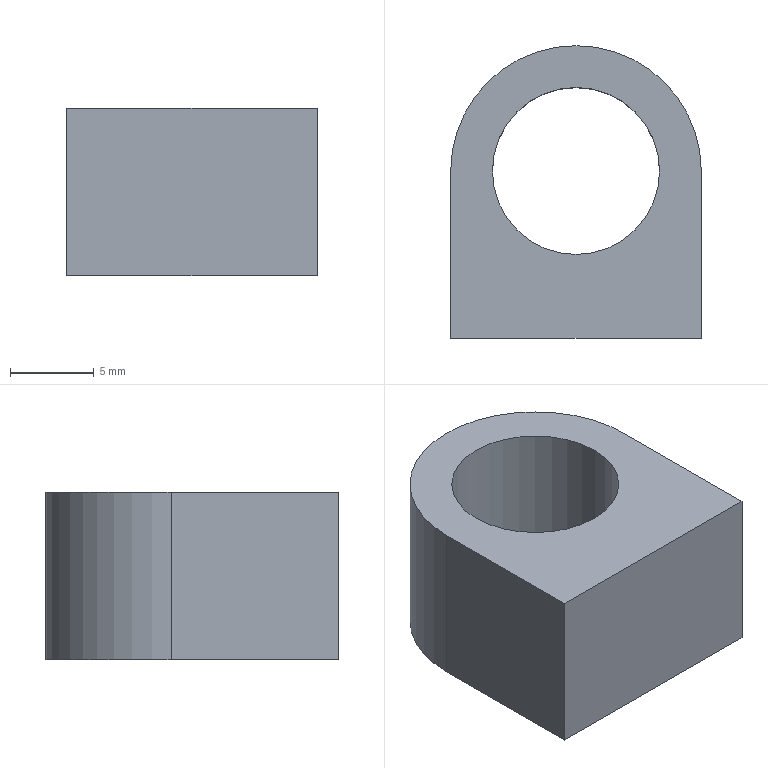Part | SolidWorks | features Extrusion 1 | 1 solid | 8 faces | box 15 x 17.5 x 10 mm | volume 1598 mm3 | plane 5 | cylinder 3 | commonest cylinder face diameters 10 x2 15 x1
STEP:
#1=CARTESIAN_POINT('',(-5.,0.,10.));
#2=VERTEX_POINT('',#1);
#3=CARTESIAN_POINT('',(5.,0.,10.));
#4=VERTEX_POINT('',#3);
#5=CARTESIAN_POINT('',(0.,0.,10.));
#6=DIRECTION('',(0.,0.,1.));
#7=DIRECTION('',(1.,0.,0.));
#8=AXIS2_PLACEMENT_3D('',#5,#6,#7);
#9=CIRCLE('',#8,5.);
#10=EDGE_CURVE('',#2,#4,#9,.T.);
#11=ORIENTED_EDGE('',*,*,#10,.T.);
#12=CARTESIAN_POINT('',(5.,0.,0.));
#13=VERTEX_POINT('',#12);
#14=CARTESIAN_POINT('',(5.,0.,10.));
#15=DIRECTION('',(0.,0.,-1.));
#16=VECTOR('',#15,1000.);
#17=LINE('',#14,#16);
#18=EDGE_CURVE('',#4,#13,#17,.T.);
#19=ORIENTED_EDGE('',*,*,#18,.T.);
#20=CARTESIAN_POINT('',(-5.,0.,0.));
#21=VERTEX_POINT('',#20);
#22=CARTESIAN_POINT('',(0.,0.,0.));
#23=DIRECTION('',(0.,0.,1.));
#24=DIRECTION('',(1.,0.,0.));
#25=AXIS2_PLACEMENT_3D('',#22,#23,#24);
#26=CIRCLE('',#25,5.);
#27=EDGE_CURVE('',#21,#13,#26,.T.);
#28=ORIENTED_EDGE('',*,*,#27,.F.);
#29=CARTESIAN_POINT('',(-5.,0.,10.));
#30=DIRECTION('',(0.,0.,-1.));
#31=VECTOR('',#30,1000.);
#32=LINE('',#29,#31);
#33=EDGE_CURVE('',#2,#21,#32,.T.);
#34=ORIENTED_EDGE('',*,*,#33,.F.);
#35=EDGE_LOOP('',(#11,#19,#28,#34));
#36=FACE_OUTER_BOUND('',#35,.T.);
#37=CARTESIAN_POINT('',(0.,0.,10.));
#38=DIRECTION('',(0.,0.,-1.));
#39=DIRECTION('',(-1.,0.,0.));
#40=AXIS2_PLACEMENT_3D('',#37,#38,#39);
#41=CYLINDRICAL_SURFACE('',#40,5.);
#42=ADVANCED_FACE('',(#36),#41,.F.);
#43=CARTESIAN_POINT('',(7.5,0.,10.));
#44=VERTEX_POINT('',#43);
#45=CARTESIAN_POINT('',(-7.5,0.,10.));
#46=VERTEX_POINT('',#45);
#47=CARTESIAN_POINT('',(0.,0.,10.));
#48=DIRECTION('',(0.,0.,1.));
#49=DIRECTION('',(1.,0.,0.));
#50=AXIS2_PLACEMENT_3D('',#47,#48,#49);
#51=CIRCLE('',#50,7.5);
#52=EDGE_CURVE('',#44,#46,#51,.T.);
#53=ORIENTED_EDGE('',*,*,#52,.T.);
#54=CARTESIAN_POINT('',(-7.5,-10.,10.));
#55=VERTEX_POINT('',#54);
#56=CARTESIAN_POINT('',(-7.5,-10.,10.));
#57=DIRECTION('',(0.,-1.,0.));
#58=VECTOR('',#57,1000.);
#59=LINE('',#56,#58);
#60=EDGE_CURVE('',#46,#55,#59,.T.);
#61=ORIENTED_EDGE('',*,*,#60,.T.);
#62=CARTESIAN_POINT('',(7.5,-10.,10.));
#63=VERTEX_POINT('',#62);
#64=CARTESIAN_POINT('',(7.5,-10.,10.));
#65=DIRECTION('',(1.,0.,0.));
#66=VECTOR('',#65,1000.);
#67=LINE('',#64,#66);
#68=EDGE_CURVE('',#55,#63,#67,.T.);
#69=ORIENTED_EDGE('',*,*,#68,.T.);
#70=CARTESIAN_POINT('',(7.5,0.,10.));
#71=DIRECTION('',(0.,1.,0.));
#72=VECTOR('',#71,1000.);
#73=LINE('',#70,#72);
#74=EDGE_CURVE('',#63,#44,#73,.T.);
#75=ORIENTED_EDGE('',*,*,#74,.T.);
#76=EDGE_LOOP('',(#53,#61,#69,#75));
#77=FACE_OUTER_BOUND('',#76,.T.);
#78=ORIENTED_EDGE('',*,*,#10,.F.);
#79=CARTESIAN_POINT('',(0.,0.,10.));
#80=DIRECTION('',(0.,0.,1.));
#81=DIRECTION('',(1.,0.,0.));
#82=AXIS2_PLACEMENT_3D('',#79,#80,#81);
#83=CIRCLE('',#82,5.);
#84=EDGE_CURVE('',#4,#2,#83,.T.);
#85=ORIENTED_EDGE('',*,*,#84,.F.);
#86=EDGE_LOOP('',(#78,#85));
#87=FACE_BOUND('',#86,.T.);
#88=CARTESIAN_POINT('',(0.,0.,10.));
#89=DIRECTION('',(0.,0.,1.));
#90=DIRECTION('',(1.,0.,0.));
#91=AXIS2_PLACEMENT_3D('',#88,#89,#90);
#92=PLANE('',#91);
#93=ADVANCED_FACE('',(#77,#87),#92,.T.);
#94=CARTESIAN_POINT('',(7.5,0.,0.));
#95=VERTEX_POINT('',#94);
#96=CARTESIAN_POINT('',(-7.5,0.,0.));
#97=VERTEX_POINT('',#96);
#98=CARTESIAN_POINT('',(0.,0.,0.));
#99=DIRECTION('',(0.,0.,1.));
#100=DIRECTION('',(1.,0.,0.));
#101=AXIS2_PLACEMENT_3D('',#98,#99,#100);
#102=CIRCLE('',#101,7.5);
#103=EDGE_CURVE('',#95,#97,#102,.T.);
#104=ORIENTED_EDGE('',*,*,#103,.F.);
#105=CARTESIAN_POINT('',(7.5,-10.,0.));
#106=VERTEX_POINT('',#105);
#107=CARTESIAN_POINT('',(7.5,0.,0.));
#108=DIRECTION('',(0.,1.,0.));
#109=VECTOR('',#108,1000.);
#110=LINE('',#107,#109);
#111=EDGE_CURVE('',#106,#95,#110,.T.);
#112=ORIENTED_EDGE('',*,*,#111,.F.);
#113=CARTESIAN_POINT('',(-7.5,-10.,0.));
#114=VERTEX_POINT('',#113);
#115=CARTESIAN_POINT('',(7.5,-10.,0.));
#116=DIRECTION('',(1.,0.,0.));
#117=VECTOR('',#116,1000.);
#118=LINE('',#115,#117);
#119=EDGE_CURVE('',#114,#106,#118,.T.);
#120=ORIENTED_EDGE('',*,*,#119,.F.);
#121=CARTESIAN_POINT('',(-7.5,-10.,0.));
#122=DIRECTION('',(0.,-1.,0.));
#123=VECTOR('',#122,1000.);
#124=LINE('',#121,#123);
#125=EDGE_CURVE('',#97,#114,#124,.T.);
#126=ORIENTED_EDGE('',*,*,#125,.F.);
#127=EDGE_LOOP('',(#104,#112,#120,#126));
#128=FACE_OUTER_BOUND('',#127,.T.);
#129=ORIENTED_EDGE('',*,*,#27,.T.);
#130=CARTESIAN_POINT('',(0.,0.,0.));
#131=DIRECTION('',(0.,0.,1.));
#132=DIRECTION('',(1.,0.,0.));
#133=AXIS2_PLACEMENT_3D('',#130,#131,#132);
#134=CIRCLE('',#133,5.);
#135=EDGE_CURVE('',#13,#21,#134,.T.);
#136=ORIENTED_EDGE('',*,*,#135,.T.);
#137=EDGE_LOOP('',(#129,#136));
#138=FACE_BOUND('',#137,.T.);
#139=CARTESIAN_POINT('',(0.,0.,0.));
#140=DIRECTION('',(0.,0.,1.));
#141=DIRECTION('',(1.,0.,0.));
#142=AXIS2_PLACEMENT_3D('',#139,#140,#141);
#143=PLANE('',#142);
#144=ADVANCED_FACE('',(#128,#138),#143,.F.);
#145=ORIENTED_EDGE('',*,*,#103,.T.);
#146=CARTESIAN_POINT('',(-7.5,0.,10.));
#147=DIRECTION('',(0.,0.,-1.));
#148=VECTOR('',#147,1000.);
#149=LINE('',#146,#148);
#150=EDGE_CURVE('',#46,#97,#149,.T.);
#151=ORIENTED_EDGE('',*,*,#150,.F.);
#152=ORIENTED_EDGE('',*,*,#52,.F.);
#153=CARTESIAN_POINT('',(7.5,0.,10.));
#154=DIRECTION('',(0.,0.,-1.));
#155=VECTOR('',#154,1000.);
#156=LINE('',#153,#155);
#157=EDGE_CURVE('',#44,#95,#156,.T.);
#158=ORIENTED_EDGE('',*,*,#157,.T.);
#159=EDGE_LOOP('',(#145,#151,#152,#158));
#160=FACE_OUTER_BOUND('',#159,.T.);
#161=CARTESIAN_POINT('',(0.,0.,10.));
#162=DIRECTION('',(0.,0.,-1.));
#163=DIRECTION('',(-1.,0.,0.));
#164=AXIS2_PLACEMENT_3D('',#161,#162,#163);
#165=CYLINDRICAL_SURFACE('',#164,7.5);
#166=ADVANCED_FACE('',(#160),#165,.T.);
#167=ORIENTED_EDGE('',*,*,#125,.T.);
#168=CARTESIAN_POINT('',(-7.5,-10.,10.));
#169=DIRECTION('',(0.,0.,-1.));
#170=VECTOR('',#169,1000.);
#171=LINE('',#168,#170);
#172=EDGE_CURVE('',#55,#114,#171,.T.);
#173=ORIENTED_EDGE('',*,*,#172,.F.);
#174=ORIENTED_EDGE('',*,*,#60,.F.);
#175=ORIENTED_EDGE('',*,*,#150,.T.);
#176=EDGE_LOOP('',(#167,#173,#174,#175));
#177=FACE_OUTER_BOUND('',#176,.T.);
#178=CARTESIAN_POINT('',(-7.5,-10.,10.));
#179=DIRECTION('',(1.,0.,0.));
#180=DIRECTION('',(0.,0.,-1.));
#181=AXIS2_PLACEMENT_3D('',#178,#179,#180);
#182=PLANE('',#181);
#183=ADVANCED_FACE('',(#177),#182,.F.);
#184=ORIENTED_EDGE('',*,*,#119,.T.);
#185=CARTESIAN_POINT('',(7.5,-10.,10.));
#186=DIRECTION('',(0.,0.,-1.));
#187=VECTOR('',#186,1000.);
#188=LINE('',#185,#187);
#189=EDGE_CURVE('',#63,#106,#188,.T.);
#190=ORIENTED_EDGE('',*,*,#189,.F.);
#191=ORIENTED_EDGE('',*,*,#68,.F.);
#192=ORIENTED_EDGE('',*,*,#172,.T.);
#193=EDGE_LOOP('',(#184,#190,#191,#192));
#194=FACE_OUTER_BOUND('',#193,.T.);
#195=CARTESIAN_POINT('',(7.5,-10.,10.));
#196=DIRECTION('',(0.,1.,0.));
#197=DIRECTION('',(0.,0.,1.));
#198=AXIS2_PLACEMENT_3D('',#195,#196,#197);
#199=PLANE('',#198);
#200=ADVANCED_FACE('',(#194),#199,.F.);
#201=ORIENTED_EDGE('',*,*,#111,.T.);
#202=ORIENTED_EDGE('',*,*,#157,.F.);
#203=ORIENTED_EDGE('',*,*,#74,.F.);
#204=ORIENTED_EDGE('',*,*,#189,.T.);
#205=EDGE_LOOP('',(#201,#202,#203,#204));
#206=FACE_OUTER_BOUND('',#205,.T.);
#207=CARTESIAN_POINT('',(7.5,0.,10.));
#208=DIRECTION('',(-1.,0.,0.));
#209=DIRECTION('',(0.,0.,1.));
#210=AXIS2_PLACEMENT_3D('',#207,#208,#209);
#211=PLANE('',#210);
#212=ADVANCED_FACE('',(#206),#211,.F.);
#213=ORIENTED_EDGE('',*,*,#18,.F.);
#214=ORIENTED_EDGE('',*,*,#84,.T.);
#215=ORIENTED_EDGE('',*,*,#33,.T.);
#216=ORIENTED_EDGE('',*,*,#135,.F.);
#217=EDGE_LOOP('',(#213,#214,#215,#216));
#218=FACE_OUTER_BOUND('',#217,.T.);
#219=CARTESIAN_POINT('',(0.,0.,10.));
#220=DIRECTION('',(0.,0.,-1.));
#221=DIRECTION('',(-1.,0.,0.));
#222=AXIS2_PLACEMENT_3D('',#219,#220,#221);
#223=CYLINDRICAL_SURFACE('',#222,5.);
#224=ADVANCED_FACE('',(#218),#223,.F.);
#225=CLOSED_SHELL('',(#42,#93,#144,#166,#183,#200,#212,#224));
#226=MANIFOLD_SOLID_BREP('',#225);
#227=CARTESIAN_POINT('',(0.,0.,0.));
#228=DIRECTION('',(0.,0.,1.));
#229=DIRECTION('',(1.,0.,0.));
#230=AXIS2_PLACEMENT_3D('',#227,#228,#229);
#231=(LENGTH_UNIT()NAMED_UNIT(*)SI_UNIT(.MILLI.,.METRE.));
#232=UNCERTAINTY_MEASURE_WITH_UNIT(LENGTH_MEASURE(0.00001),#231,'','');
#233=(NAMED_UNIT(*)PLANE_ANGLE_UNIT()SI_UNIT($,.RADIAN.));
#234=(NAMED_UNIT(*)SI_UNIT($,.STERADIAN.)SOLID_ANGLE_UNIT());
#235=(GEOMETRIC_REPRESENTATION_CONTEXT(3)GLOBAL_UNCERTAINTY_ASSIGNED_CONTEXT((#232))GLOBAL_UNIT_ASSIGNED_CONTEXT((#231,#233,#234))REPRESENTATION_CONTEXT('',''));
#236=ADVANCED_BREP_SHAPE_REPRESENTATION('',(#226,#230),#235);